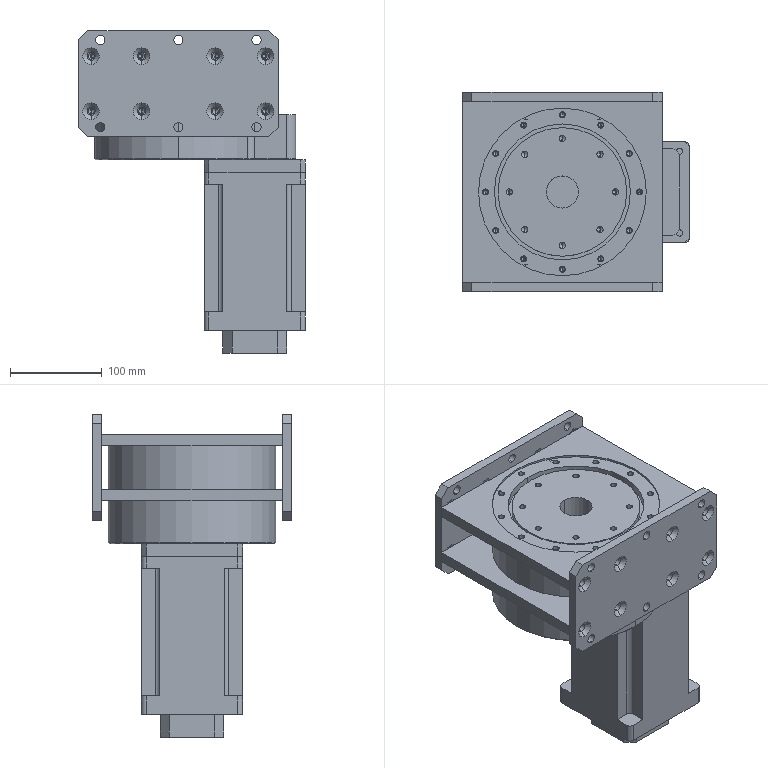Part | SolidWorks | features InContextFeatHolder 2, CompositeCurve 1 | 11 solids | 825 faces | box 246.625 x 216.5 x 351 mm | volume 5460860 mm3 | cylinder 558 | cone 130 | plane 125 | torus 12 | commonest cylinder face diameters 27.5 x114 6.6 x74 6.8 x64 65.623 x55 71.25 x55 9 x48